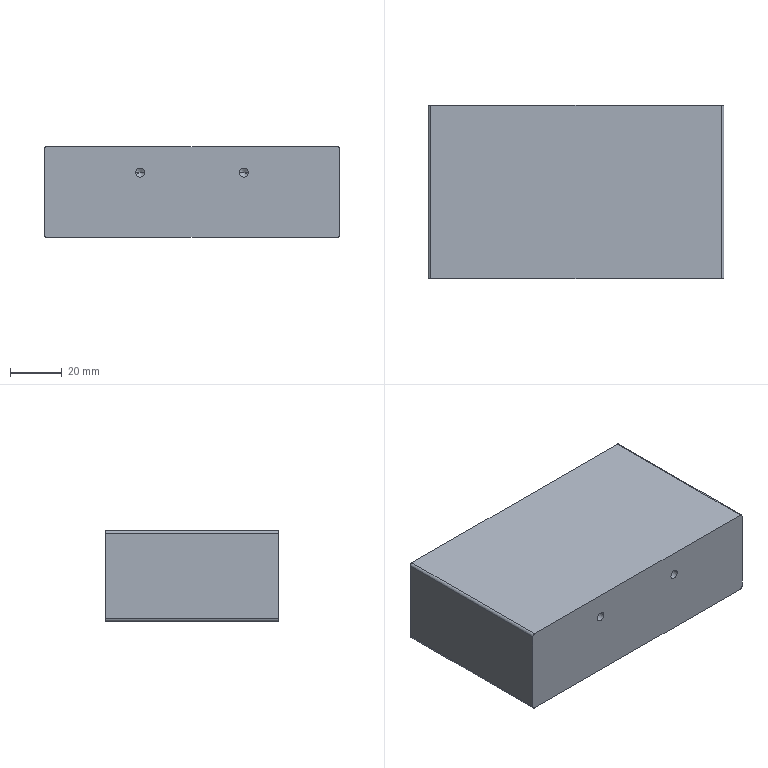NC program | NX | posted with a generic post | part box 114 x 67 x 35 mm
Whole program:
N10 G17 G21 G94 G90
(DRILLING_COPY , TOOL : D4A45)
N12 T02 M6
N14 G54
N16 G17 G0 G90 X20. Y-7.5 B0. C0. S5000 M3
N18 G43 Z30. H2
N20 G94 G81 G98 Z-1. F250. R3.
N22 X-20.
N24 G80
N26 G0 X-20. Y-7.5 Z30.
N28 M5
(DRILLING_COPY_COPY_COPY_COPY_COPY_COPY , TOOL : 3.5ZT)
N30 T15 M6
N32 G54
N34 G17 G0 G90 X20. Y-7.5 B0. C0. S1910 M3
N36 G43 Z30. H15
N38 G94 G83 G98 Z-11.552 F180. Q2. R3.
N40 X-20.
N42 G80
N44 G0 X-20. Y-7.5 Z30.
N46 M5
N48 M2